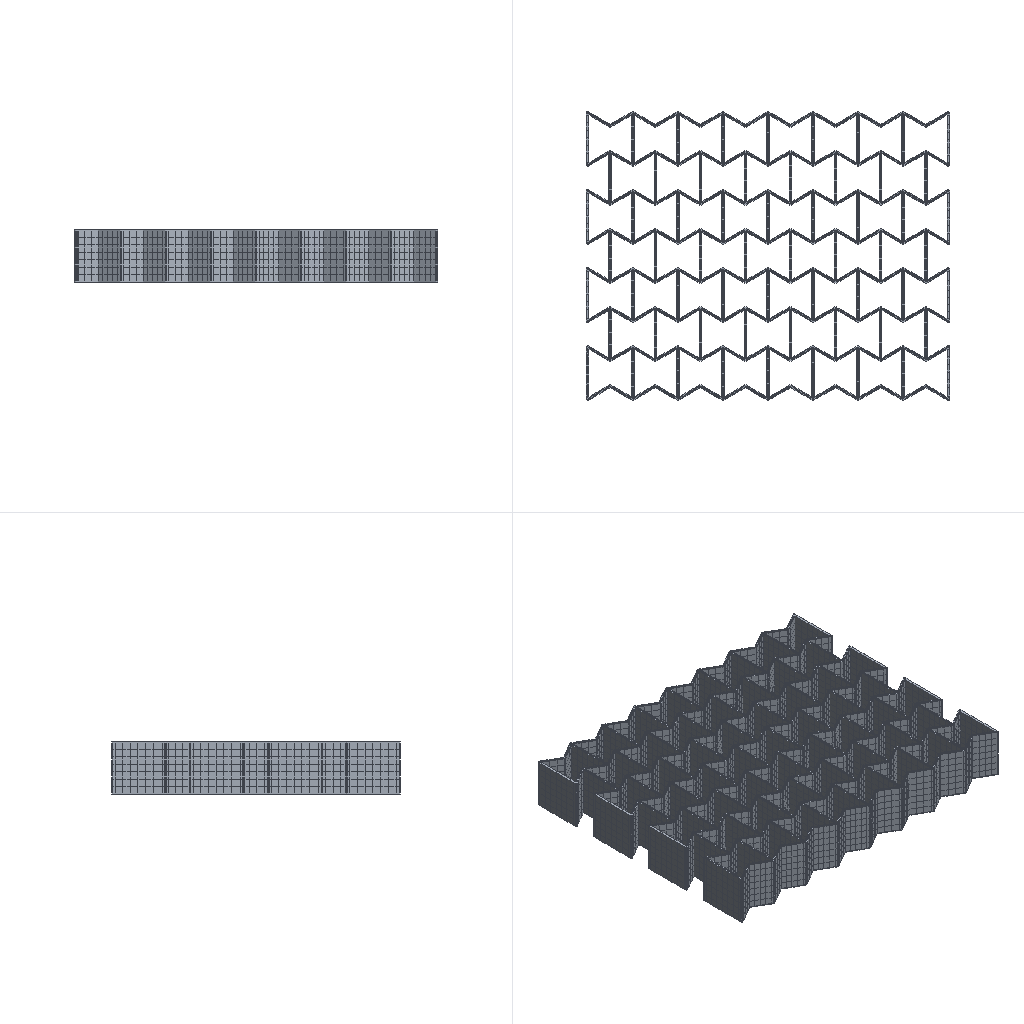Simulation study | abaqus
Set-up summary:
category,name,step,type,value,unit,region
solver,abaqus
solver,version,,,Abaqus/Explicit 2020
units,not stated in the deck,,not stated
analysis,deck,,transient,transient
load_step,Step-1,Step-1,transient
load_step,requested,,,1
mesh,nodes,,,45264
mesh,elements,,,33215
element_type,C3D8R,,solid,33215
load,load commands in deck,,count,2
bc,support commands in deck,,count,12
material,MATERIAL-1,,in results
check,setup vs results,,match,"per instance, exact: element labels, types and connectivity; labels of the nodes the elements use; coordinates of those nodes at SINGLE_PRECISION in 1 of 1 instance(s)"
Abaqus input file, long lists of numbers shortened:
*Heading
** Job name: Job-2 Model name: Model-1
** Generated by: Abaqus/CAE 2020
*Preprint, echo=NO, model=NO, history=NO, contact=NO
**
** PARTS
**
*Part, name=work
*Node
      1,  -73.112,  -31.634,          20.
      2,  -74.112,  -31.634,          20.
** (45262 more lines like these left out)
*Element, type=C3D8R
    1,   990,     3,     2,     1,  6648,  5661,  5660,  5659
    2,   989,   985,     3,   990,  6647,  6643,  5661,  6648
** (33213 more lines like these left out)
*Nset, nset=Set-2, generate
     1,  45264,      1
*Elset, elset=Set-2, generate
     1,  33215,      1
** Section: Section-1
*Solid Section, elset=Set-2, material=Material-1
,
*End Part
**
**
** ASSEMBLY
**
*Assembly, name=Assembly
**
*Instance, name=work-1, part=work
*End Instance
**
*Node
      1,   65.452,         -7.5,          10.
*Node
      2,  -74.112,         -7.5,          10.
*Nset, nset=Set-1, instance=work-1
     2,     3,     8,    13,    19,    25,    83,    84,   100,   122,   142,   153,   154,   170,   183,   210
   234,   261,   464,   465,   497,   532,   564,   601,  1002,  1003,  1004,  1243,  1244,  1245,  1463,  1464
** (16 more lines like these left out)
*Elset, elset=Set-1, instance=work-1
     1,     6,    28,    29,    30,    31,    47,    69,   323,   403,   490,   492,   494,   496,   618,   653
   714,   763,   925,   926,   927,  1035,  1036,  1151,  2204,  2349,  2518,  2519,  2520,  2521,  2665,  2828
** (12 more lines like these left out)
*Nset, nset=Set-3
 1,
*Nset, nset=Set-5
 2,
*Nset, nset=m_Set-2
 1,
*Nset, nset=m_Set-4
 2,
*Elset, elset=_s_Surf-1_S3, internal, instance=work-1
  3900,  4109,  4583,  4727,  8645,  8854,  9328,  9472, 13390, 13599, 14073, 14217, 18135, 18344, 18818, 18962
 22880, 23089, 23563, 23707, 27625, 27834, 28308, 28452, 32370, 32579, 33053, 33197
*Elset, elset=_s_Surf-1_S6, internal, instance=work-1
  3700,  3852,  3853,  3854,  3855,  4029,  4127,  4128,  4129,  4130,  4386,  4463,  4718,  4728,  4729,  8445
  8597,  8598,  8599,  8600,  8774,  8872,  8873,  8874,  8875,  9131,  9208,  9463,  9473,  9474, 13190, 13342
** (5 more lines like these left out)
*Elset, elset=_s_Surf-1_S4, internal, instance=work-1
  3984,  3985,  4122,  4218,  4526,  4527,  4528,  4529,  4578,  4736,  4743,  4744,  4745,  8729,  8730,  8867
  8963,  9271,  9272,  9273,  9274,  9323,  9481,  9488,  9489,  9490, 13474, 13475, 13612, 13708, 14016, 14017
** (4 more lines like these left out)
*Surface, type=ELEMENT, name=s_Surf-1
_s_Surf-1_S3, S3
_s_Surf-1_S6, S6
_s_Surf-1_S4, S4
*Elset, elset=_s_Surf-2_S3, internal, instance=work-1
   323,   653,   714,  2204,  5068,  5398,  5459,  6949,  9813, 10143, 10204, 11694, 14558, 14888, 14949, 16439
 19303, 19633, 19694, 21184, 24048, 24378, 24439, 25929, 28793, 29123, 29184, 30674
*Elset, elset=_s_Surf-2_S6, internal, instance=work-1
    47,    69,   403,  1035,  1036,  1151,  2665,  2828,  4792,  4814,  5148,  5780,  5781,  5896,  7410,  7573
  9537,  9559,  9893, 10525, 10526, 10641, 12155, 12318, 14282, 14304, 14638, 15270, 15271, 15386, 16900, 17063
** (2 more lines like these left out)
*Elset, elset=_s_Surf-2_S4, internal, instance=work-1
     1,     6,    28,    29,    30,    31,   490,   492,   494,   496,   618,   763,   925,   926,   927,  2349
  2518,  2519,  2520,  2521,  4746,  4751,  4773,  4774,  4775,  4776,  5235,  5237,  5239,  5241,  5363,  5508
** (7 more lines like these left out)
*Surface, type=ELEMENT, name=s_Surf-2
_s_Surf-2_S3, S3
_s_Surf-2_S6, S6
_s_Surf-2_S4, S4
** Constraint: Constraint-1
*Coupling, constraint name=Constraint-1, ref node=m_Set-2, surface=s_Surf-1
*Kinematic
** Constraint: Constraint-2
*Coupling, constraint name=Constraint-2, ref node=m_Set-4, surface=s_Surf-2
*Kinematic
*End Assembly
*Amplitude, name=Amp-1
             0.,              0.,            0.01,              1.
**
** MATERIALS
**
*Material, name=Material-1
*Density
 2.7e-09,
*Elastic
72000., 0.28
*Plastic
289.,0.
**
** INTERACTION PROPERTIES
**
*Surface Interaction, name=IntProp-1
*Friction
 0.15,
*Surface Behavior, pressure-overclosure=HARD
** ----------------------------------------------------------------
**
** STEP: Step-1
**
*Step, name=Step-1, nlgeom=YES
*Dynamic, Explicit
, 0.01
*Bulk Viscosity
0.06, 1.2
** Mass Scaling: Semi-Automatic
**               Whole Model
*Fixed Mass Scaling, factor=500.
**
** BOUNDARY CONDITIONS
**
** Name: BC-2 Type: 位移/转角
*Boundary, amplitude=Amp-1
Set-3, 1, 1, -35.
Set-3, 2, 2
Set-3, 3, 3
Set-3, 4, 4
Set-3, 5, 5
Set-3, 6, 6
** Name: BC-3 Type: 位移/转角
*Boundary, amplitude=Amp-1
Set-5, 1, 1, 35.
Set-5, 2, 2
Set-5, 3, 3
Set-5, 4, 4
Set-5, 5, 5
Set-5, 6, 6
**
** INTERACTIONS
**
** Interaction: Int-1
*Contact, op=NEW
*Contact Inclusions, ALL EXTERIOR
*Contact Property Assignment
 ,  , IntProp-1
**
** OUTPUT REQUESTS
**
*Restart, write, number interval=1, time marks=NO
**
** FIELD OUTPUT: F-Output-1
**
*Output, field, number interval=50
*Node Output
A, CF, RF, RM, RT, U, V
*Element Output, directions=YES
E, EVF, LE, MISES, MISESMAX, PE, PEEQ, PEEQVAVG, PEVAVG, S, SEQUT, SVAVG, YIELDPOT
*Contact Output
CDISP, CSTRESS
**
** HISTORY OUTPUT: H-Output-1
**
*Output, history, time interval=5e-07
*Node Output, nset=Set-3
RF1, U1
*End Step
Results summary:
result,step,Step-1,completed,increments=59285 time=0.01/0.01
result,analysis,,,transient
result,last_loadstep,,,1
result,primary field,,,U
result,reaction total,,FX,2757.15,model units
result,reaction total,,FY,-697.178,model units
result,reaction total,,FZ,-247.68,model units